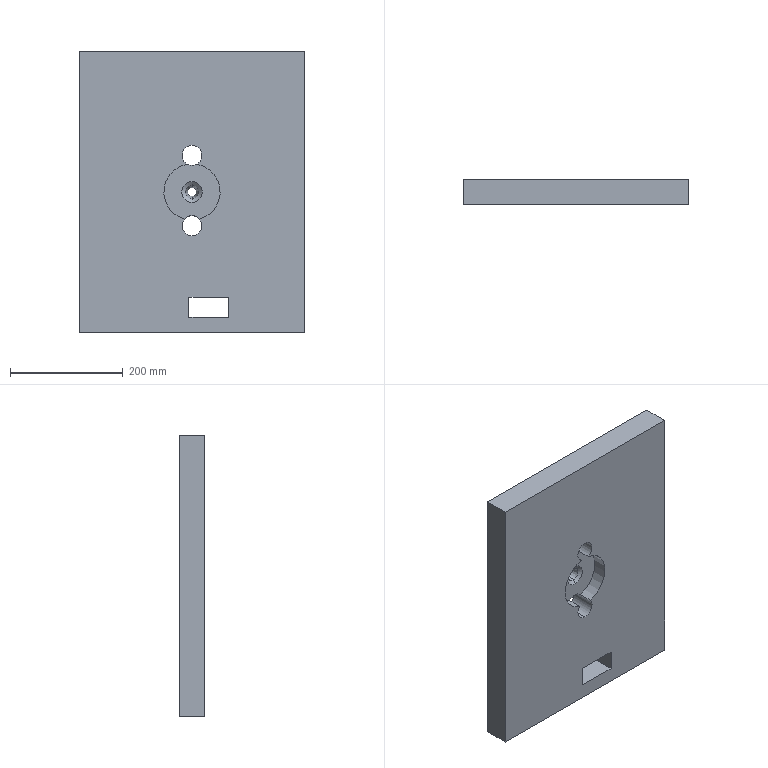Part | STEP file | 1 solid | 21 faces | box 400 x 45 x 500 mm | volume 8595426 mm3 | plane 11 | cylinder 6 | cone 4 | commonest cylinder face diameters 35.5 x4 100 x2